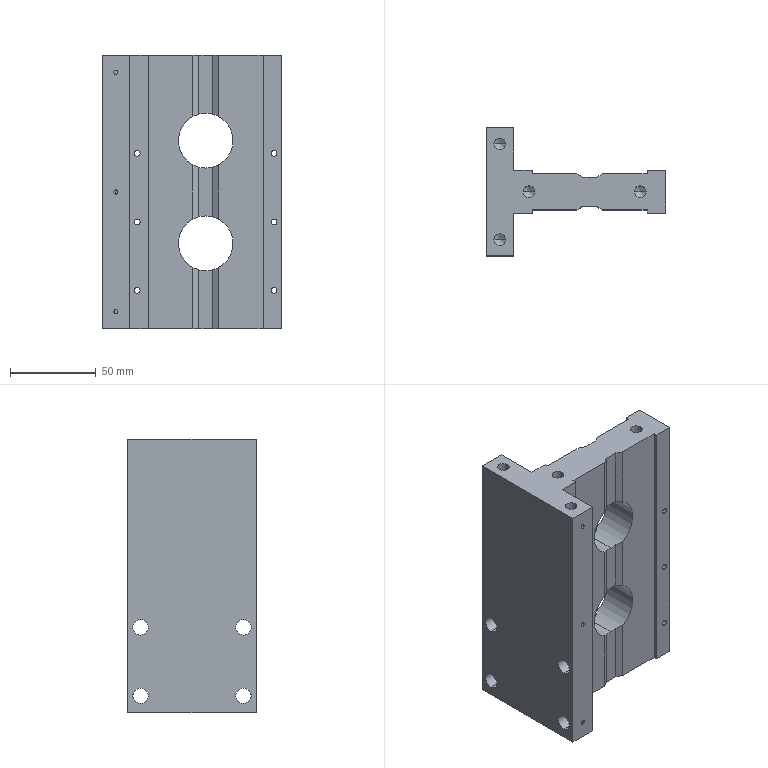Part | STEP file | Fixed seat | 1 solid | 114 faces | box 105 x 75 x 160 mm | volume 453829 mm3 | cylinder 56 | plane 42 | cone 16 | commonest cylinder face diameters 2.5 x12 3.3 x12 6.8 x8 9 x8 13.5 x8 5 x4